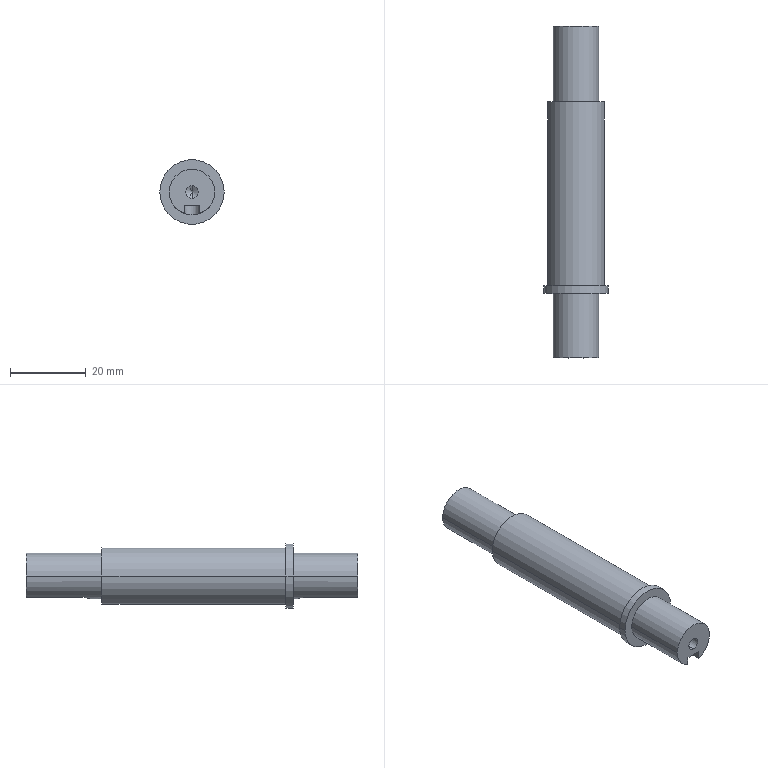Part | SolidWorks | features ICE 3, HoleWzd 2, RefAxis 1, Revolution 1 | 1 solid | 29 faces | box 17 x 87.5 x 17 mm | volume 12724 mm3 | cylinder 14 | plane 11 | cone 4 | commonest cylinder face diameters 3.3 x4 12 x4 4 x2 15 x2 17 x2
STEP:
#1=CARTESIAN_POINT('',(0.,60.4,-1.65));
#2=VERTEX_POINT('',#1);
#3=CARTESIAN_POINT('',(0.,60.4,1.65));
#4=VERTEX_POINT('',#3);
#5=CARTESIAN_POINT('',(0.,60.4,0.));
#6=DIRECTION('',(0.,1.,0.));
#7=DIRECTION('',(0.,0.,1.));
#8=AXIS2_PLACEMENT_3D('',#5,#6,#7);
#9=CIRCLE('',#8,1.65);
#10=EDGE_CURVE('',#2,#4,#9,.T.);
#11=ORIENTED_EDGE('',*,*,#10,.F.);
#12=CARTESIAN_POINT('',(0.,70.5,-1.65));
#13=VERTEX_POINT('',#12);
#14=CARTESIAN_POINT('',(0.,70.5,-1.65));
#15=DIRECTION('',(0.,1.,0.));
#16=VECTOR('',#15,1000.);
#17=LINE('',#14,#16);
#18=EDGE_CURVE('',#2,#13,#17,.T.);
#19=ORIENTED_EDGE('',*,*,#18,.T.);
#20=CARTESIAN_POINT('',(0.,70.5,1.65));
#21=VERTEX_POINT('',#20);
#22=CARTESIAN_POINT('',(0.,70.5,0.));
#23=DIRECTION('',(0.,1.,0.));
#24=DIRECTION('',(0.,0.,1.));
#25=AXIS2_PLACEMENT_3D('',#22,#23,#24);
#26=CIRCLE('',#25,1.65);
#27=EDGE_CURVE('',#13,#21,#26,.T.);
#28=ORIENTED_EDGE('',*,*,#27,.T.);
#29=CARTESIAN_POINT('',(0.,70.5,1.65));
#30=DIRECTION('',(0.,1.,0.));
#31=VECTOR('',#30,1000.);
#32=LINE('',#29,#31);
#33=EDGE_CURVE('',#4,#21,#32,.T.);
#34=ORIENTED_EDGE('',*,*,#33,.F.);
#35=EDGE_LOOP('',(#11,#19,#28,#34));
#36=FACE_OUTER_BOUND('',#35,.T.);
#37=CARTESIAN_POINT('',(0.,70.5,0.));
#38=DIRECTION('',(0.,1.,0.));
#39=DIRECTION('',(0.,0.,1.));
#40=AXIS2_PLACEMENT_3D('',#37,#38,#39);
#41=CYLINDRICAL_SURFACE('',#40,1.65);
#42=ADVANCED_FACE('',(#36),#41,.F.);
#43=CARTESIAN_POINT('',(0.,59.409,0.));
#44=VERTEX_POINT('',#43);
#45=CARTESIAN_POINT('',(0.,60.4,1.65));
#46=DIRECTION('',(0.,0.515,0.8572));
#47=VECTOR('',#46,1000.);
#48=LINE('',#45,#47);
#49=EDGE_CURVE('',#44,#4,#48,.T.);
#50=ORIENTED_EDGE('',*,*,#49,.F.);
#51=CARTESIAN_POINT('',(0.,60.4,-1.65));
#52=DIRECTION('',(0.,0.515,-0.8572));
#53=VECTOR('',#52,1000.);
#54=LINE('',#51,#53);
#55=EDGE_CURVE('',#44,#2,#54,.T.);
#56=ORIENTED_EDGE('',*,*,#55,.T.);
#57=ORIENTED_EDGE('',*,*,#10,.T.);
#58=EDGE_LOOP('',(#50,#56,#57));
#59=FACE_OUTER_BOUND('',#58,.T.);
#60=CARTESIAN_POINT('',(0.,60.4,0.));
#61=DIRECTION('',(0.,1.,0.));
#62=DIRECTION('',(0.,0.,1.));
#63=AXIS2_PLACEMENT_3D('',#60,#61,#62);
#64=CONICAL_SURFACE('',#63,1.65,1.03);
#65=ADVANCED_FACE('',(#59),#64,.F.);
#66=CARTESIAN_POINT('',(0.,-6.9,1.65));
#67=VERTEX_POINT('',#66);
#68=CARTESIAN_POINT('',(0.,-6.9,-1.65));
#69=VERTEX_POINT('',#68);
#70=CARTESIAN_POINT('',(0.,-6.9,0.));
#71=DIRECTION('',(0.,-1.,0.));
#72=DIRECTION('',(0.,0.,-1.));
#73=AXIS2_PLACEMENT_3D('',#70,#71,#72);
#74=CIRCLE('',#73,1.65);
#75=EDGE_CURVE('',#67,#69,#74,.T.);
#76=ORIENTED_EDGE('',*,*,#75,.F.);
#77=CARTESIAN_POINT('',(0.,-17.,1.65));
#78=VERTEX_POINT('',#77);
#79=CARTESIAN_POINT('',(0.,-17.,1.65));
#80=DIRECTION('',(0.,-1.,0.));
#81=VECTOR('',#80,1000.);
#82=LINE('',#79,#81);
#83=EDGE_CURVE('',#67,#78,#82,.T.);
#84=ORIENTED_EDGE('',*,*,#83,.T.);
#85=CARTESIAN_POINT('',(0.,-17.,-1.65));
#86=VERTEX_POINT('',#85);
#87=CARTESIAN_POINT('',(0.,-17.,0.));
#88=DIRECTION('',(0.,-1.,0.));
#89=DIRECTION('',(0.,0.,-1.));
#90=AXIS2_PLACEMENT_3D('',#87,#88,#89);
#91=CIRCLE('',#90,1.65);
#92=EDGE_CURVE('',#78,#86,#91,.T.);
#93=ORIENTED_EDGE('',*,*,#92,.T.);
#94=CARTESIAN_POINT('',(0.,-17.,-1.65));
#95=DIRECTION('',(0.,-1.,0.));
#96=VECTOR('',#95,1000.);
#97=LINE('',#94,#96);
#98=EDGE_CURVE('',#69,#86,#97,.T.);
#99=ORIENTED_EDGE('',*,*,#98,.F.);
#100=EDGE_LOOP('',(#76,#84,#93,#99));
#101=FACE_OUTER_BOUND('',#100,.T.);
#102=CARTESIAN_POINT('',(0.,-17.,0.));
#103=DIRECTION('',(0.,-1.,0.));
#104=DIRECTION('',(0.,0.,-1.));
#105=AXIS2_PLACEMENT_3D('',#102,#103,#104);
#106=CYLINDRICAL_SURFACE('',#105,1.65);
#107=ADVANCED_FACE('',(#101),#106,.F.);
#108=CARTESIAN_POINT('',(0.,-5.909,0.));
#109=VERTEX_POINT('',#108);
#110=CARTESIAN_POINT('',(0.,-6.9,-1.65));
#111=DIRECTION('',(0.,-0.515,-0.8572));
#112=VECTOR('',#111,1000.);
#113=LINE('',#110,#112);
#114=EDGE_CURVE('',#109,#69,#113,.T.);
#115=ORIENTED_EDGE('',*,*,#114,.F.);
#116=CARTESIAN_POINT('',(0.,-6.9,1.65));
#117=DIRECTION('',(0.,-0.515,0.8572));
#118=VECTOR('',#117,1000.);
#119=LINE('',#116,#118);
#120=EDGE_CURVE('',#109,#67,#119,.T.);
#121=ORIENTED_EDGE('',*,*,#120,.T.);
#122=ORIENTED_EDGE('',*,*,#75,.T.);
#123=EDGE_LOOP('',(#115,#121,#122));
#124=FACE_OUTER_BOUND('',#123,.T.);
#125=CARTESIAN_POINT('',(0.,-6.9,0.));
#126=DIRECTION('',(0.,-1.,0.));
#127=DIRECTION('',(0.,0.,-1.));
#128=AXIS2_PLACEMENT_3D('',#125,#126,#127);
#129=CONICAL_SURFACE('',#128,1.65,1.03);
#130=ADVANCED_FACE('',(#124),#129,.F.);
#131=CARTESIAN_POINT('',(6.,-17.,0.));
#132=VERTEX_POINT('',#131);
#133=CARTESIAN_POINT('',(-6.,-17.,0.));
#134=VERTEX_POINT('',#133);
#135=CARTESIAN_POINT('',(0.,-17.,0.));
#136=DIRECTION('',(0.,-1.,0.));
#137=DIRECTION('',(1.,0.,0.));
#138=AXIS2_PLACEMENT_3D('',#135,#136,#137);
#139=CIRCLE('',#138,6.);
#140=EDGE_CURVE('',#132,#134,#139,.T.);
#141=ORIENTED_EDGE('',*,*,#140,.F.);
#142=CARTESIAN_POINT('',(6.,0.,0.));
#143=VERTEX_POINT('',#142);
#144=CARTESIAN_POINT('',(6.,-17.,0.));
#145=DIRECTION('',(0.,1.,0.));
#146=VECTOR('',#145,1000.);
#147=LINE('',#144,#146);
#148=EDGE_CURVE('',#132,#143,#147,.T.);
#149=ORIENTED_EDGE('',*,*,#148,.T.);
#150=CARTESIAN_POINT('',(-6.,0.,0.));
#151=VERTEX_POINT('',#150);
#152=CARTESIAN_POINT('',(0.,0.,0.));
#153=DIRECTION('',(0.,-1.,0.));
#154=DIRECTION('',(1.,0.,0.));
#155=AXIS2_PLACEMENT_3D('',#152,#153,#154);
#156=CIRCLE('',#155,6.);
#157=EDGE_CURVE('',#143,#151,#156,.T.);
#158=ORIENTED_EDGE('',*,*,#157,.T.);
#159=CARTESIAN_POINT('',(-6.,-17.,0.));
#160=DIRECTION('',(0.,1.,0.));
#161=VECTOR('',#160,1000.);
#162=LINE('',#159,#161);
#163=EDGE_CURVE('',#134,#151,#162,.T.);
#164=ORIENTED_EDGE('',*,*,#163,.F.);
#165=EDGE_LOOP('',(#141,#149,#158,#164));
#166=FACE_OUTER_BOUND('',#165,.T.);
#167=CARTESIAN_POINT('',(0.,-17.,0.));
#168=DIRECTION('',(0.,1.,0.));
#169=DIRECTION('',(-1.,0.,0.));
#170=AXIS2_PLACEMENT_3D('',#167,#168,#169);
#171=CYLINDRICAL_SURFACE('',#170,6.);
#172=ADVANCED_FACE('',(#166),#171,.T.);
#173=CARTESIAN_POINT('',(8.5,2.,0.));
#174=VERTEX_POINT('',#173);
#175=CARTESIAN_POINT('',(-8.5,2.,0.));
#176=VERTEX_POINT('',#175);
#177=CARTESIAN_POINT('',(0.,2.,0.));
#178=DIRECTION('',(0.,-1.,0.));
#179=DIRECTION('',(1.,0.,0.));
#180=AXIS2_PLACEMENT_3D('',#177,#178,#179);
#181=CIRCLE('',#180,8.5);
#182=EDGE_CURVE('',#174,#176,#181,.T.);
#183=ORIENTED_EDGE('',*,*,#182,.T.);
#184=CARTESIAN_POINT('',(-8.5,0.,0.));
#185=VERTEX_POINT('',#184);
#186=CARTESIAN_POINT('',(-8.5,0.,0.));
#187=DIRECTION('',(0.,-1.,0.));
#188=VECTOR('',#187,1000.);
#189=LINE('',#186,#188);
#190=EDGE_CURVE('',#176,#185,#189,.T.);
#191=ORIENTED_EDGE('',*,*,#190,.T.);
#192=CARTESIAN_POINT('',(8.5,0.,0.));
#193=VERTEX_POINT('',#192);
#194=CARTESIAN_POINT('',(0.,0.,0.));
#195=DIRECTION('',(0.,-1.,0.));
#196=DIRECTION('',(1.,0.,0.));
#197=AXIS2_PLACEMENT_3D('',#194,#195,#196);
#198=CIRCLE('',#197,8.5);
#199=EDGE_CURVE('',#193,#185,#198,.T.);
#200=ORIENTED_EDGE('',*,*,#199,.F.);
#201=CARTESIAN_POINT('',(8.5,0.,0.));
#202=DIRECTION('',(0.,-1.,0.));
#203=VECTOR('',#202,1000.);
#204=LINE('',#201,#203);
#205=EDGE_CURVE('',#174,#193,#204,.T.);
#206=ORIENTED_EDGE('',*,*,#205,.F.);
#207=EDGE_LOOP('',(#183,#191,#200,#206));
#208=FACE_OUTER_BOUND('',#207,.T.);
#209=CARTESIAN_POINT('',(0.,0.,0.));
#210=DIRECTION('',(0.,-1.,0.));
#211=DIRECTION('',(1.,0.,0.));
#212=AXIS2_PLACEMENT_3D('',#209,#210,#211);
#213=CYLINDRICAL_SURFACE('',#212,8.5);
#214=ADVANCED_FACE('',(#208),#213,.T.);
#215=CARTESIAN_POINT('',(7.5,50.5,0.));
#216=VERTEX_POINT('',#215);
#217=CARTESIAN_POINT('',(-7.5,50.5,0.));
#218=VERTEX_POINT('',#217);
#219=CARTESIAN_POINT('',(0.,50.5,0.));
#220=DIRECTION('',(0.,-1.,0.));
#221=DIRECTION('',(1.,0.,0.));
#222=AXIS2_PLACEMENT_3D('',#219,#220,#221);
#223=CIRCLE('',#222,7.5);
#224=EDGE_CURVE('',#216,#218,#223,.T.);
#225=ORIENTED_EDGE('',*,*,#224,.T.);
#226=CARTESIAN_POINT('',(-7.5,2.,0.));
#227=VERTEX_POINT('',#226);
#228=CARTESIAN_POINT('',(-7.5,0.,0.));
#229=DIRECTION('',(0.,-1.,0.));
#230=VECTOR('',#229,1000.);
#231=LINE('',#228,#230);
#232=EDGE_CURVE('',#218,#227,#231,.T.);
#233=ORIENTED_EDGE('',*,*,#232,.T.);
#234=CARTESIAN_POINT('',(7.5,2.,0.));
#235=VERTEX_POINT('',#234);
#236=CARTESIAN_POINT('',(0.,2.,0.));
#237=DIRECTION('',(0.,-1.,0.));
#238=DIRECTION('',(1.,0.,0.));
#239=AXIS2_PLACEMENT_3D('',#236,#237,#238);
#240=CIRCLE('',#239,7.5);
#241=EDGE_CURVE('',#235,#227,#240,.T.);
#242=ORIENTED_EDGE('',*,*,#241,.F.);
#243=CARTESIAN_POINT('',(7.5,0.,0.));
#244=DIRECTION('',(0.,-1.,0.));
#245=VECTOR('',#244,1000.);
#246=LINE('',#243,#245);
#247=EDGE_CURVE('',#216,#235,#246,.T.);
#248=ORIENTED_EDGE('',*,*,#247,.F.);
#249=EDGE_LOOP('',(#225,#233,#242,#248));
#250=FACE_OUTER_BOUND('',#249,.T.);
#251=CARTESIAN_POINT('',(0.,0.,0.));
#252=DIRECTION('',(0.,-1.,0.));
#253=DIRECTION('',(1.,0.,0.));
#254=AXIS2_PLACEMENT_3D('',#251,#252,#253);
#255=CYLINDRICAL_SURFACE('',#254,7.5);
#256=ADVANCED_FACE('',(#250),#255,.T.);
#257=CARTESIAN_POINT('',(6.,70.5,0.));
#258=VERTEX_POINT('',#257);
#259=CARTESIAN_POINT('',(-6.,70.5,0.));
#260=VERTEX_POINT('',#259);
#261=CARTESIAN_POINT('',(0.,70.5,0.));
#262=DIRECTION('',(0.,-1.,0.));
#263=DIRECTION('',(1.,0.,0.));
#264=AXIS2_PLACEMENT_3D('',#261,#262,#263);
#265=CIRCLE('',#264,6.);
#266=EDGE_CURVE('',#258,#260,#265,.T.);
#267=ORIENTED_EDGE('',*,*,#266,.T.);
#268=CARTESIAN_POINT('',(-6.,50.5,0.));
#269=VERTEX_POINT('',#268);
#270=CARTESIAN_POINT('',(-6.,0.,0.));
#271=DIRECTION('',(0.,-1.,0.));
#272=VECTOR('',#271,1000.);
#273=LINE('',#270,#272);
#274=EDGE_CURVE('',#260,#269,#273,.T.);
#275=ORIENTED_EDGE('',*,*,#274,.T.);
#276=CARTESIAN_POINT('',(6.,50.5,0.));
#277=VERTEX_POINT('',#276);
#278=CARTESIAN_POINT('',(0.,50.5,0.));
#279=DIRECTION('',(0.,-1.,0.));
#280=DIRECTION('',(1.,0.,0.));
#281=AXIS2_PLACEMENT_3D('',#278,#279,#280);
#282=CIRCLE('',#281,6.);
#283=EDGE_CURVE('',#277,#269,#282,.T.);
#284=ORIENTED_EDGE('',*,*,#283,.F.);
#285=CARTESIAN_POINT('',(6.,0.,0.));
#286=DIRECTION('',(0.,-1.,0.));
#287=VECTOR('',#286,1000.);
#288=LINE('',#285,#287);
#289=EDGE_CURVE('',#258,#277,#288,.T.);
#290=ORIENTED_EDGE('',*,*,#289,.F.);
#291=EDGE_LOOP('',(#267,#275,#284,#290));
#292=FACE_OUTER_BOUND('',#291,.T.);
#293=CARTESIAN_POINT('',(0.,0.,0.));
#294=DIRECTION('',(0.,-1.,0.));
#295=DIRECTION('',(1.,0.,0.));
#296=AXIS2_PLACEMENT_3D('',#293,#294,#295);
#297=CYLINDRICAL_SURFACE('',#296,6.);
#298=ADVANCED_FACE('',(#292),#297,.T.);
#299=CARTESIAN_POINT('',(0.,0.,0.));
#300=DIRECTION('',(0.,-1.,0.));
#301=DIRECTION('',(1.,0.,0.));
#302=AXIS2_PLACEMENT_3D('',#299,#300,#301);
#303=CIRCLE('',#302,6.);
#304=EDGE_CURVE('',#151,#143,#303,.T.);
#305=ORIENTED_EDGE('',*,*,#304,.F.);
#306=ORIENTED_EDGE('',*,*,#157,.F.);
#307=EDGE_LOOP('',(#305,#306));
#308=FACE_BOUND('',#307,.T.);
#309=ORIENTED_EDGE('',*,*,#199,.T.);
#310=CARTESIAN_POINT('',(0.,0.,0.));
#311=DIRECTION('',(0.,-1.,0.));
#312=DIRECTION('',(1.,0.,0.));
#313=AXIS2_PLACEMENT_3D('',#310,#311,#312);
#314=CIRCLE('',#313,8.5);
#315=EDGE_CURVE('',#185,#193,#314,.T.);
#316=ORIENTED_EDGE('',*,*,#315,.T.);
#317=EDGE_LOOP('',(#309,#316));
#318=FACE_OUTER_BOUND('',#317,.T.);
#319=CARTESIAN_POINT('',(-8.5,0.,0.));
#320=DIRECTION('',(0.,1.,0.));
#321=DIRECTION('',(-1.,0.,0.));
#322=AXIS2_PLACEMENT_3D('',#319,#320,#321);
#323=PLANE('',#322);
#324=ADVANCED_FACE('',(#308,#318),#323,.F.);
#325=CARTESIAN_POINT('',(0.,70.5,0.));
#326=DIRECTION('',(0.,1.,0.));
#327=DIRECTION('',(0.,0.,1.));
#328=AXIS2_PLACEMENT_3D('',#325,#326,#327);
#329=CIRCLE('',#328,1.65);
#330=EDGE_CURVE('',#21,#13,#329,.T.);
#331=ORIENTED_EDGE('',*,*,#330,.F.);
#332=ORIENTED_EDGE('',*,*,#27,.F.);
#333=EDGE_LOOP('',(#331,#332));
#334=FACE_BOUND('',#333,.T.);
#335=CARTESIAN_POINT('',(-2.,70.5,-3.5));
#336=VERTEX_POINT('',#335);
#337=CARTESIAN_POINT('',(2.,70.5,-3.5));
#338=VERTEX_POINT('',#337);
#339=CARTESIAN_POINT('',(0.,70.5,-3.5));
#340=DIRECTION('',(1.,0.,0.));
#341=VECTOR('',#340,1000.);
#342=LINE('',#339,#341);
#343=EDGE_CURVE('',#336,#338,#342,.T.);
#344=ORIENTED_EDGE('',*,*,#343,.F.);
#345=CARTESIAN_POINT('',(-2.,70.5,-5.657));
#346=VERTEX_POINT('',#345);
#347=CARTESIAN_POINT('',(-2.,70.5,0.));
#348=DIRECTION('',(0.,0.,-1.));
#349=VECTOR('',#348,1000.);
#350=LINE('',#347,#349);
#351=EDGE_CURVE('',#336,#346,#350,.T.);
#352=ORIENTED_EDGE('',*,*,#351,.T.);
#353=CARTESIAN_POINT('',(0.,70.5,0.));
#354=DIRECTION('',(0.,-1.,0.));
#355=DIRECTION('',(1.,0.,0.));
#356=AXIS2_PLACEMENT_3D('',#353,#354,#355);
#357=CIRCLE('',#356,6.);
#358=EDGE_CURVE('',#260,#346,#357,.T.);
#359=ORIENTED_EDGE('',*,*,#358,.F.);
#360=ORIENTED_EDGE('',*,*,#266,.F.);
#361=CARTESIAN_POINT('',(2.,70.5,-5.657));
#362=VERTEX_POINT('',#361);
#363=CARTESIAN_POINT('',(0.,70.5,0.));
#364=DIRECTION('',(0.,-1.,0.));
#365=DIRECTION('',(1.,0.,0.));
#366=AXIS2_PLACEMENT_3D('',#363,#364,#365);
#367=CIRCLE('',#366,6.);
#368=EDGE_CURVE('',#362,#258,#367,.T.);
#369=ORIENTED_EDGE('',*,*,#368,.F.);
#370=CARTESIAN_POINT('',(2.,70.5,0.));
#371=DIRECTION('',(0.,0.,1.));
#372=VECTOR('',#371,1000.);
#373=LINE('',#370,#372);
#374=EDGE_CURVE('',#362,#338,#373,.T.);
#375=ORIENTED_EDGE('',*,*,#374,.T.);
#376=EDGE_LOOP('',(#344,#352,#359,#360,#369,#375));
#377=FACE_OUTER_BOUND('',#376,.T.);
#378=CARTESIAN_POINT('',(0.,70.5,0.));
#379=DIRECTION('',(0.,-1.,0.));
#380=DIRECTION('',(1.,0.,0.));
#381=AXIS2_PLACEMENT_3D('',#378,#379,#380);
#382=PLANE('',#381);
#383=ADVANCED_FACE('',(#334,#377),#382,.F.);
#384=ORIENTED_EDGE('',*,*,#274,.F.);
#385=ORIENTED_EDGE('',*,*,#358,.T.);
#386=CARTESIAN_POINT('',(-2.,55.5,-5.657));
#387=VERTEX_POINT('',#386);
#388=CARTESIAN_POINT('',(-2.,0.,-5.657));
#389=DIRECTION('',(0.,-1.,0.));
#390=VECTOR('',#389,1000.);
#391=LINE('',#388,#390);
#392=EDGE_CURVE('',#346,#387,#391,.T.);
#393=ORIENTED_EDGE('',*,*,#392,.T.);
#394=CARTESIAN_POINT('',(2.,55.5,-5.657));
#395=VERTEX_POINT('',#394);
#396=CARTESIAN_POINT('',(-2.,55.5,-5.657));
#397=CARTESIAN_POINT('',(-2.,55.367,-5.657));
#398=CARTESIAN_POINT('',(-1.987,55.236,-5.662));
#399=CARTESIAN_POINT('',(-1.935,54.979,-5.679));
#400=CARTESIAN_POINT('',(-1.897,54.852,-5.693));
#401=CARTESIAN_POINT('',(-1.796,54.61,-5.725));
#402=CARTESIAN_POINT('',(-1.735,54.496,-5.744));
#403=CARTESIAN_POINT('',(-1.59,54.279,-5.786));
#404=CARTESIAN_POINT('',(-1.506,54.177,-5.809));
#405=CARTESIAN_POINT('',(-1.231,53.903,-5.875));
#406=CARTESIAN_POINT('',(-1.01,53.754,-5.919));
#407=CARTESIAN_POINT('',(-0.6496,53.604,-5.966));
#408=CARTESIAN_POINT('',(-0.5226,53.565,-5.979));
#409=CARTESIAN_POINT('',(-0.264,53.513,-5.996));
#410=CARTESIAN_POINT('',(-0.1336,53.5,-6.));
#411=CARTESIAN_POINT('',(0.1294,53.5,-6.));
#412=CARTESIAN_POINT('',(0.2629,53.513,-5.996));
#413=CARTESIAN_POINT('',(0.5202,53.564,-5.979));
#414=CARTESIAN_POINT('',(0.6454,53.602,-5.966));
#415=CARTESIAN_POINT('',(0.8889,53.704,-5.935));
#416=CARTESIAN_POINT('',(1.004,53.766,-5.916));
#417=CARTESIAN_POINT('',(1.22,53.91,-5.876));
#418=CARTESIAN_POINT('',(1.322,53.993,-5.853));
#419=CARTESIAN_POINT('',(1.506,54.177,-5.809));
#420=CARTESIAN_POINT('',(1.588,54.277,-5.787));
#421=CARTESIAN_POINT('',(1.733,54.493,-5.745));
#422=CARTESIAN_POINT('',(1.796,54.61,-5.725));
#423=CARTESIAN_POINT('',(1.946,54.971,-5.677));
#424=CARTESIAN_POINT('',(2.,55.234,-5.657));
#425=CARTESIAN_POINT('',(2.,55.5,-5.657));
#426=B_SPLINE_CURVE_WITH_KNOTS('',3,(#396,#397,#398,#399,#400,#401,#402,#403,#404,#405,#406,#407,#408,#409,#410,#411,#412,#413,#414,#415,#416,#417,#418,#419,#420,#421,#422,#423,#424,#425),.UNSPECIFIED.,.F.,.F.,(4,2,2,2,2,2,2,2,2,2,2,2,2,2,4),(0.,0.0003935,0.000787,0.00118,0.001574,0.002361,0.002754,0.003148,0.003541,0.003935,0.004328,0.004722,0.005115,0.005509,0.006296),.UNSPECIFIED.);
#427=EDGE_CURVE('',#387,#395,#426,.T.);
#428=ORIENTED_EDGE('',*,*,#427,.T.);
#429=CARTESIAN_POINT('',(2.,0.,-5.657));
#430=DIRECTION('',(0.,1.,0.));
#431=VECTOR('',#430,1000.);
#432=LINE('',#429,#431);
#433=EDGE_CURVE('',#395,#362,#432,.T.);
#434=ORIENTED_EDGE('',*,*,#433,.T.);
#435=ORIENTED_EDGE('',*,*,#368,.T.);
#436=ORIENTED_EDGE('',*,*,#289,.T.);
#437=CARTESIAN_POINT('',(0.,50.5,0.));
#438=DIRECTION('',(0.,-1.,0.));
#439=DIRECTION('',(1.,0.,0.));
#440=AXIS2_PLACEMENT_3D('',#437,#438,#439);
#441=CIRCLE('',#440,6.);
#442=EDGE_CURVE('',#269,#277,#441,.T.);
#443=ORIENTED_EDGE('',*,*,#442,.F.);
#444=EDGE_LOOP('',(#384,#385,#393,#428,#434,#435,#436,#443));
#445=FACE_OUTER_BOUND('',#444,.T.);
#446=CARTESIAN_POINT('',(0.,0.,0.));
#447=DIRECTION('',(0.,-1.,0.));
#448=DIRECTION('',(1.,0.,0.));
#449=AXIS2_PLACEMENT_3D('',#446,#447,#448);
#450=CYLINDRICAL_SURFACE('',#449,6.);
#451=ADVANCED_FACE('',(#445),#450,.T.);
#452=ORIENTED_EDGE('',*,*,#224,.F.);
#453=CARTESIAN_POINT('',(0.,50.5,0.));
#454=DIRECTION('',(0.,-1.,0.));
#455=DIRECTION('',(1.,0.,0.));
#456=AXIS2_PLACEMENT_3D('',#453,#454,#455);
#457=CIRCLE('',#456,7.5);
#458=EDGE_CURVE('',#218,#216,#457,.T.);
#459=ORIENTED_EDGE('',*,*,#458,.F.);
#460=EDGE_LOOP('',(#452,#459));
#461=FACE_OUTER_BOUND('',#460,.T.);
#462=ORIENTED_EDGE('',*,*,#283,.T.);
#463=ORIENTED_EDGE('',*,*,#442,.T.);
#464=EDGE_LOOP('',(#462,#463));
#465=FACE_BOUND('',#464,.T.);
#466=CARTESIAN_POINT('',(-6.,50.5,0.));
#467=DIRECTION('',(0.,-1.,0.));
#468=DIRECTION('',(1.,0.,0.));
#469=AXIS2_PLACEMENT_3D('',#466,#467,#468);
#470=PLANE('',#469);
#471=ADVANCED_FACE('',(#461,#465),#470,.F.);
#472=ORIENTED_EDGE('',*,*,#232,.F.);
#473=ORIENTED_EDGE('',*,*,#458,.T.);
#474=ORIENTED_EDGE('',*,*,#247,.T.);
#475=CARTESIAN_POINT('',(0.,2.,0.));
#476=DIRECTION('',(0.,-1.,0.));
#477=DIRECTION('',(1.,0.,0.));
#478=AXIS2_PLACEMENT_3D('',#475,#476,#477);
#479=CIRCLE('',#478,7.5);
#480=EDGE_CURVE('',#227,#235,#479,.T.);
#481=ORIENTED_EDGE('',*,*,#480,.F.);
#482=EDGE_LOOP('',(#472,#473,#474,#481));
#483=FACE_OUTER_BOUND('',#482,.T.);
#484=CARTESIAN_POINT('',(0.,0.,0.));
#485=DIRECTION('',(0.,-1.,0.));
#486=DIRECTION('',(1.,0.,0.));
#487=AXIS2_PLACEMENT_3D('',#484,#485,#486);
#488=CYLINDRICAL_SURFACE('',#487,7.5);
#489=ADVANCED_FACE('',(#483),#488,.T.);
#490=ORIENTED_EDGE('',*,*,#182,.F.);
#491=CARTESIAN_POINT('',(0.,2.,0.));
#492=DIRECTION('',(0.,-1.,0.));
#493=DIRECTION('',(1.,0.,0.));
#494=AXIS2_PLACEMENT_3D('',#491,#492,#493);
#495=CIRCLE('',#494,8.5);
#496=EDGE_CURVE('',#176,#174,#495,.T.);
#497=ORIENTED_EDGE('',*,*,#496,.F.);
#498=EDGE_LOOP('',(#490,#497));
#499=FACE_OUTER_BOUND('',#498,.T.);
#500=ORIENTED_EDGE('',*,*,#241,.T.);
#501=ORIENTED_EDGE('',*,*,#480,.T.);
#502=EDGE_LOOP('',(#500,#501));
#503=FACE_BOUND('',#502,.T.);
#504=CARTESIAN_POINT('',(-7.5,2.,0.));
#505=DIRECTION('',(0.,-1.,0.));
#506=DIRECTION('',(1.,0.,0.));
#507=AXIS2_PLACEMENT_3D('',#504,#505,#506);
#508=PLANE('',#507);
#509=ADVANCED_FACE('',(#499,#503),#508,.F.);
#510=ORIENTED_EDGE('',*,*,#190,.F.);
#511=ORIENTED_EDGE('',*,*,#496,.T.);
#512=ORIENTED_EDGE('',*,*,#205,.T.);
#513=ORIENTED_EDGE('',*,*,#315,.F.);
#514=EDGE_LOOP('',(#510,#511,#512,#513));
#515=FACE_OUTER_BOUND('',#514,.T.);
#516=CARTESIAN_POINT('',(0.,0.,0.));
#517=DIRECTION('',(0.,-1.,0.));
#518=DIRECTION('',(1.,0.,0.));
#519=AXIS2_PLACEMENT_3D('',#516,#517,#518);
#520=CYLINDRICAL_SURFACE('',#519,8.5);
#521=ADVANCED_FACE('',(#515),#520,.T.);
#522=ORIENTED_EDGE('',*,*,#148,.F.);
#523=CARTESIAN_POINT('',(2.,-17.,-5.657));
#524=VERTEX_POINT('',#523);
#525=CARTESIAN_POINT('',(0.,-17.,0.));
#526=DIRECTION('',(0.,-1.,0.));
#527=DIRECTION('',(1.,0.,0.));
#528=AXIS2_PLACEMENT_3D('',#525,#526,#527);
#529=CIRCLE('',#528,6.);
#530=EDGE_CURVE('',#524,#132,#529,.T.);
#531=ORIENTED_EDGE('',*,*,#530,.F.);
#532=CARTESIAN_POINT('',(2.,-3.,-5.657));
#533=VERTEX_POINT('',#532);
#534=CARTESIAN_POINT('',(2.,-17.,-5.657));
#535=DIRECTION('',(0.,1.,0.));
#536=VECTOR('',#535,1000.);
#537=LINE('',#534,#536);
#538=EDGE_CURVE('',#524,#533,#537,.T.);
#539=ORIENTED_EDGE('',*,*,#538,.T.);
#540=CARTESIAN_POINT('',(-2.,-3.,-5.657));
#541=VERTEX_POINT('',#540);
#542=CARTESIAN_POINT('',(2.,-3.,-5.657));
#543=CARTESIAN_POINT('',(2.,-2.867,-5.657));
#544=CARTESIAN_POINT('',(1.987,-2.736,-5.662));
#545=CARTESIAN_POINT('',(1.935,-2.479,-5.679));
#546=CARTESIAN_POINT('',(1.897,-2.352,-5.693));
#547=CARTESIAN_POINT('',(1.796,-2.11,-5.725));
#548=CARTESIAN_POINT('',(1.735,-1.996,-5.744));
#549=CARTESIAN_POINT('',(1.59,-1.779,-5.786));
#550=CARTESIAN_POINT('',(1.506,-1.677,-5.809));
#551=CARTESIAN_POINT('',(1.231,-1.403,-5.875));
#552=CARTESIAN_POINT('',(1.01,-1.254,-5.919));
#553=CARTESIAN_POINT('',(0.6496,-1.104,-5.966));
#554=CARTESIAN_POINT('',(0.5226,-1.065,-5.979));
#555=CARTESIAN_POINT('',(0.264,-1.013,-5.996));
#556=CARTESIAN_POINT('',(0.1336,-1.,-6.));
#557=CARTESIAN_POINT('',(-0.1294,-0.9999,-6.));
#558=CARTESIAN_POINT('',(-0.2629,-1.013,-5.996));
#559=CARTESIAN_POINT('',(-0.5202,-1.064,-5.979));
#560=CARTESIAN_POINT('',(-0.6454,-1.102,-5.966));
#561=CARTESIAN_POINT('',(-0.8889,-1.204,-5.935));
#562=CARTESIAN_POINT('',(-1.004,-1.266,-5.916));
#563=CARTESIAN_POINT('',(-1.22,-1.41,-5.876));
#564=CARTESIAN_POINT('',(-1.322,-1.493,-5.853));
#565=CARTESIAN_POINT('',(-1.506,-1.677,-5.809));
#566=CARTESIAN_POINT('',(-1.588,-1.777,-5.787));
#567=CARTESIAN_POINT('',(-1.733,-1.993,-5.745));
#568=CARTESIAN_POINT('',(-1.796,-2.11,-5.725));
#569=CARTESIAN_POINT('',(-1.946,-2.471,-5.677));
#570=CARTESIAN_POINT('',(-2.,-2.734,-5.657));
#571=CARTESIAN_POINT('',(-2.,-3.,-5.657));
#572=B_SPLINE_CURVE_WITH_KNOTS('',3,(#542,#543,#544,#545,#546,#547,#548,#549,#550,#551,#552,#553,#554,#555,#556,#557,#558,#559,#560,#561,#562,#563,#564,#565,#566,#567,#568,#569,#570,#571),.UNSPECIFIED.,.F.,.F.,(4,2,2,2,2,2,2,2,2,2,2,2,2,2,4),(0.,0.0003935,0.000787,0.00118,0.001574,0.002361,0.002754,0.003148,0.003541,0.003935,0.004328,0.004722,0.005115,0.005509,0.006296),.UNSPECIFIED.);
#573=EDGE_CURVE('',#533,#541,#572,.T.);
#574=ORIENTED_EDGE('',*,*,#573,.T.);
#575=CARTESIAN_POINT('',(-2.,-17.,-5.657));
#576=VERTEX_POINT('',#575);
#577=CARTESIAN_POINT('',(-2.,-17.,-5.657));
#578=DIRECTION('',(0.,-1.,0.));
#579=VECTOR('',#578,1000.);
#580=LINE('',#577,#579);
#581=EDGE_CURVE('',#541,#576,#580,.T.);
#582=ORIENTED_EDGE('',*,*,#581,.T.);
#583=CARTESIAN_POINT('',(0.,-17.,0.));
#584=DIRECTION('',(0.,-1.,0.));
#585=DIRECTION('',(1.,0.,0.));
#586=AXIS2_PLACEMENT_3D('',#583,#584,#585);
#587=CIRCLE('',#586,6.);
#588=EDGE_CURVE('',#134,#576,#587,.T.);
#589=ORIENTED_EDGE('',*,*,#588,.F.);
#590=ORIENTED_EDGE('',*,*,#163,.T.);
#591=ORIENTED_EDGE('',*,*,#304,.T.);
#592=EDGE_LOOP('',(#522,#531,#539,#574,#582,#589,#590,#591));
#593=FACE_OUTER_BOUND('',#592,.T.);
#594=CARTESIAN_POINT('',(0.,-17.,0.));
#595=DIRECTION('',(0.,1.,0.));
#596=DIRECTION('',(-1.,0.,0.));
#597=AXIS2_PLACEMENT_3D('',#594,#595,#596);
#598=CYLINDRICAL_SURFACE('',#597,6.);
#599=ADVANCED_FACE('',(#593),#598,.T.);
#600=CARTESIAN_POINT('',(0.,-17.,0.));
#601=DIRECTION('',(0.,-1.,0.));
#602=DIRECTION('',(0.,0.,-1.));
#603=AXIS2_PLACEMENT_3D('',#600,#601,#602);
#604=CIRCLE('',#603,1.65);
#605=EDGE_CURVE('',#86,#78,#604,.T.);
#606=ORIENTED_EDGE('',*,*,#605,.F.);
#607=ORIENTED_EDGE('',*,*,#92,.F.);
#608=EDGE_LOOP('',(#606,#607));
#609=FACE_BOUND('',#608,.T.);
#610=CARTESIAN_POINT('',(2.,-17.,-3.5));
#611=VERTEX_POINT('',#610);
#612=CARTESIAN_POINT('',(2.,-17.,0.));
#613=DIRECTION('',(0.,0.,1.));
#614=VECTOR('',#613,1000.);
#615=LINE('',#612,#614);
#616=EDGE_CURVE('',#524,#611,#615,.T.);
#617=ORIENTED_EDGE('',*,*,#616,.F.);
#618=ORIENTED_EDGE('',*,*,#530,.T.);
#619=ORIENTED_EDGE('',*,*,#140,.T.);
#620=ORIENTED_EDGE('',*,*,#588,.T.);
#621=CARTESIAN_POINT('',(-2.,-17.,-3.5));
#622=VERTEX_POINT('',#621);
#623=CARTESIAN_POINT('',(-2.,-17.,0.));
#624=DIRECTION('',(0.,0.,-1.));
#625=VECTOR('',#624,1000.);
#626=LINE('',#623,#625);
#627=EDGE_CURVE('',#622,#576,#626,.T.);
#628=ORIENTED_EDGE('',*,*,#627,.F.);
#629=CARTESIAN_POINT('',(0.,-17.,-3.5));
#630=DIRECTION('',(1.,0.,0.));
#631=VECTOR('',#630,1000.);
#632=LINE('',#629,#631);
#633=EDGE_CURVE('',#622,#611,#632,.T.);
#634=ORIENTED_EDGE('',*,*,#633,.T.);
#635=EDGE_LOOP('',(#617,#618,#619,#620,#628,#634));
#636=FACE_OUTER_BOUND('',#635,.T.);
#637=CARTESIAN_POINT('',(0.,-17.,0.));
#638=DIRECTION('',(0.,-1.,0.));
#639=DIRECTION('',(1.,0.,0.));
#640=AXIS2_PLACEMENT_3D('',#637,#638,#639);
#641=PLANE('',#640);
#642=ADVANCED_FACE('',(#609,#636),#641,.T.);
#643=ORIENTED_EDGE('',*,*,#343,.T.);
#644=CARTESIAN_POINT('',(2.,55.5,-3.5));
#645=VERTEX_POINT('',#644);
#646=CARTESIAN_POINT('',(2.,71.5,-3.5));
#647=DIRECTION('',(0.,-1.,0.));
#648=VECTOR('',#647,1000.);
#649=LINE('',#646,#648);
#650=EDGE_CURVE('',#338,#645,#649,.T.);
#651=ORIENTED_EDGE('',*,*,#650,.T.);
#652=CARTESIAN_POINT('',(-2.,55.5,-3.5));
#653=VERTEX_POINT('',#652);
#654=CARTESIAN_POINT('',(0.,55.5,-3.5));
#655=DIRECTION('',(0.,0.,-1.));
#656=DIRECTION('',(-1.,0.,0.));
#657=AXIS2_PLACEMENT_3D('',#654,#655,#656);
#658=CIRCLE('',#657,2.);
#659=EDGE_CURVE('',#645,#653,#658,.T.);
#660=ORIENTED_EDGE('',*,*,#659,.T.);
#661=CARTESIAN_POINT('',(-2.,71.5,-3.5));
#662=DIRECTION('',(0.,1.,0.));
#663=VECTOR('',#662,1000.);
#664=LINE('',#661,#663);
#665=EDGE_CURVE('',#653,#336,#664,.T.);
#666=ORIENTED_EDGE('',*,*,#665,.T.);
#667=EDGE_LOOP('',(#643,#651,#660,#666));
#668=FACE_OUTER_BOUND('',#667,.T.);
#669=CARTESIAN_POINT('',(0.,71.5,-3.5));
#670=DIRECTION('',(0.,0.,-1.));
#671=DIRECTION('',(-1.,0.,0.));
#672=AXIS2_PLACEMENT_3D('',#669,#670,#671);
#673=PLANE('',#672);
#674=ADVANCED_FACE('',(#668),#673,.T.);
#675=ORIENTED_EDGE('',*,*,#665,.F.);
#676=CARTESIAN_POINT('',(-2.,55.5,-3.5));
#677=DIRECTION('',(0.,0.,-1.));
#678=VECTOR('',#677,1000.);
#679=LINE('',#676,#678);
#680=EDGE_CURVE('',#653,#387,#679,.T.);
#681=ORIENTED_EDGE('',*,*,#680,.T.);
#682=ORIENTED_EDGE('',*,*,#392,.F.);
#683=ORIENTED_EDGE('',*,*,#351,.F.);
#684=EDGE_LOOP('',(#675,#681,#682,#683));
#685=FACE_OUTER_BOUND('',#684,.T.);
#686=CARTESIAN_POINT('',(-2.,71.5,-3.5));
#687=DIRECTION('',(-1.,0.,0.));
#688=DIRECTION('',(0.,0.,1.));
#689=AXIS2_PLACEMENT_3D('',#686,#687,#688);
#690=PLANE('',#689);
#691=ADVANCED_FACE('',(#685),#690,.F.);
#692=ORIENTED_EDGE('',*,*,#680,.F.);
#693=ORIENTED_EDGE('',*,*,#659,.F.);
#694=CARTESIAN_POINT('',(2.,55.5,-3.5));
#695=DIRECTION('',(0.,0.,-1.));
#696=VECTOR('',#695,1000.);
#697=LINE('',#694,#696);
#698=EDGE_CURVE('',#645,#395,#697,.T.);
#699=ORIENTED_EDGE('',*,*,#698,.T.);
#700=ORIENTED_EDGE('',*,*,#427,.F.);
#701=EDGE_LOOP('',(#692,#693,#699,#700));
#702=FACE_OUTER_BOUND('',#701,.T.);
#703=CARTESIAN_POINT('',(0.,55.5,-3.5));
#704=DIRECTION('',(0.,0.,-1.));
#705=DIRECTION('',(-1.,0.,0.));
#706=AXIS2_PLACEMENT_3D('',#703,#704,#705);
#707=CYLINDRICAL_SURFACE('',#706,2.);
#708=ADVANCED_FACE('',(#702),#707,.F.);
#709=ORIENTED_EDGE('',*,*,#433,.F.);
#710=ORIENTED_EDGE('',*,*,#698,.F.);
#711=ORIENTED_EDGE('',*,*,#650,.F.);
#712=ORIENTED_EDGE('',*,*,#374,.F.);
#713=EDGE_LOOP('',(#709,#710,#711,#712));
#714=FACE_OUTER_BOUND('',#713,.T.);
#715=CARTESIAN_POINT('',(2.,71.5,-3.5));
#716=DIRECTION('',(1.,0.,0.));
#717=DIRECTION('',(0.,0.,-1.));
#718=AXIS2_PLACEMENT_3D('',#715,#716,#717);
#719=PLANE('',#718);
#720=ADVANCED_FACE('',(#714),#719,.F.);
#721=CARTESIAN_POINT('',(2.,-3.,-3.5));
#722=VERTEX_POINT('',#721);
#723=CARTESIAN_POINT('',(2.,-3.,-3.5));
#724=DIRECTION('',(0.,0.,-1.));
#725=VECTOR('',#724,1000.);
#726=LINE('',#723,#725);
#727=EDGE_CURVE('',#722,#533,#726,.T.);
#728=ORIENTED_EDGE('',*,*,#727,.F.);
#729=CARTESIAN_POINT('',(-2.,-3.,-3.5));
#730=VERTEX_POINT('',#729);
#731=CARTESIAN_POINT('',(0.,-3.,-3.5));
#732=DIRECTION('',(0.,0.,-1.));
#733=DIRECTION('',(-1.,0.,0.));
#734=AXIS2_PLACEMENT_3D('',#731,#732,#733);
#735=CIRCLE('',#734,2.);
#736=EDGE_CURVE('',#730,#722,#735,.T.);
#737=ORIENTED_EDGE('',*,*,#736,.F.);
#738=CARTESIAN_POINT('',(-2.,-3.,-3.5));
#739=DIRECTION('',(0.,0.,-1.));
#740=VECTOR('',#739,1000.);
#741=LINE('',#738,#740);
#742=EDGE_CURVE('',#730,#541,#741,.T.);
#743=ORIENTED_EDGE('',*,*,#742,.T.);
#744=ORIENTED_EDGE('',*,*,#573,.F.);
#745=EDGE_LOOP('',(#728,#737,#743,#744));
#746=FACE_OUTER_BOUND('',#745,.T.);
#747=CARTESIAN_POINT('',(0.,-3.,-3.5));
#748=DIRECTION('',(0.,0.,-1.));
#749=DIRECTION('',(-1.,0.,0.));
#750=AXIS2_PLACEMENT_3D('',#747,#748,#749);
#751=CYLINDRICAL_SURFACE('',#750,2.);
#752=ADVANCED_FACE('',(#746),#751,.F.);
#753=ORIENTED_EDGE('',*,*,#616,.T.);
#754=CARTESIAN_POINT('',(2.,-18.,-3.5));
#755=DIRECTION('',(0.,-1.,0.));
#756=VECTOR('',#755,1000.);
#757=LINE('',#754,#756);
#758=EDGE_CURVE('',#722,#611,#757,.T.);
#759=ORIENTED_EDGE('',*,*,#758,.F.);
#760=ORIENTED_EDGE('',*,*,#727,.T.);
#761=ORIENTED_EDGE('',*,*,#538,.F.);
#762=EDGE_LOOP('',(#753,#759,#760,#761));
#763=FACE_OUTER_BOUND('',#762,.T.);
#764=CARTESIAN_POINT('',(2.,-18.,-3.5));
#765=DIRECTION('',(1.,0.,0.));
#766=DIRECTION('',(0.,0.,-1.));
#767=AXIS2_PLACEMENT_3D('',#764,#765,#766);
#768=PLANE('',#767);
#769=ADVANCED_FACE('',(#763),#768,.F.);
#770=ORIENTED_EDGE('',*,*,#742,.F.);
#771=CARTESIAN_POINT('',(-2.,-18.,-3.5));
#772=DIRECTION('',(0.,1.,0.));
#773=VECTOR('',#772,1000.);
#774=LINE('',#771,#773);
#775=EDGE_CURVE('',#622,#730,#774,.T.);
#776=ORIENTED_EDGE('',*,*,#775,.F.);
#777=ORIENTED_EDGE('',*,*,#627,.T.);
#778=ORIENTED_EDGE('',*,*,#581,.F.);
#779=EDGE_LOOP('',(#770,#776,#777,#778));
#780=FACE_OUTER_BOUND('',#779,.T.);
#781=CARTESIAN_POINT('',(-2.,-18.,-3.5));
#782=DIRECTION('',(-1.,0.,0.));
#783=DIRECTION('',(0.,0.,1.));
#784=AXIS2_PLACEMENT_3D('',#781,#782,#783);
#785=PLANE('',#784);
#786=ADVANCED_FACE('',(#780),#785,.F.);
#787=ORIENTED_EDGE('',*,*,#775,.T.);
#788=ORIENTED_EDGE('',*,*,#736,.T.);
#789=ORIENTED_EDGE('',*,*,#758,.T.);
#790=ORIENTED_EDGE('',*,*,#633,.F.);
#791=EDGE_LOOP('',(#787,#788,#789,#790));
#792=FACE_OUTER_BOUND('',#791,.T.);
#793=CARTESIAN_POINT('',(0.,-18.,-3.5));
#794=DIRECTION('',(0.,0.,-1.));
#795=DIRECTION('',(-1.,0.,0.));
#796=AXIS2_PLACEMENT_3D('',#793,#794,#795);
#797=PLANE('',#796);
#798=ADVANCED_FACE('',(#792),#797,.T.);
#799=ORIENTED_EDGE('',*,*,#120,.F.);
#800=ORIENTED_EDGE('',*,*,#114,.T.);
#801=CARTESIAN_POINT('',(0.,-6.9,0.));
#802=DIRECTION('',(0.,-1.,0.));
#803=DIRECTION('',(0.,0.,-1.));
#804=AXIS2_PLACEMENT_3D('',#801,#802,#803);
#805=CIRCLE('',#804,1.65);
#806=EDGE_CURVE('',#69,#67,#805,.T.);
#807=ORIENTED_EDGE('',*,*,#806,.T.);
#808=EDGE_LOOP('',(#799,#800,#807));
#809=FACE_OUTER_BOUND('',#808,.T.);
#810=CARTESIAN_POINT('',(0.,-6.9,0.));
#811=DIRECTION('',(0.,-1.,0.));
#812=DIRECTION('',(0.,0.,-1.));
#813=AXIS2_PLACEMENT_3D('',#810,#811,#812);
#814=CONICAL_SURFACE('',#813,1.65,1.03);
#815=ADVANCED_FACE('',(#809),#814,.F.);
#816=ORIENTED_EDGE('',*,*,#83,.F.);
#817=ORIENTED_EDGE('',*,*,#806,.F.);
#818=ORIENTED_EDGE('',*,*,#98,.T.);
#819=ORIENTED_EDGE('',*,*,#605,.T.);
#820=EDGE_LOOP('',(#816,#817,#818,#819));
#821=FACE_OUTER_BOUND('',#820,.T.);
#822=CARTESIAN_POINT('',(0.,-17.,0.));
#823=DIRECTION('',(0.,-1.,0.));
#824=DIRECTION('',(0.,0.,-1.));
#825=AXIS2_PLACEMENT_3D('',#822,#823,#824);
#826=CYLINDRICAL_SURFACE('',#825,1.65);
#827=ADVANCED_FACE('',(#821),#826,.F.);
#828=ORIENTED_EDGE('',*,*,#55,.F.);
#829=ORIENTED_EDGE('',*,*,#49,.T.);
#830=CARTESIAN_POINT('',(0.,60.4,0.));
#831=DIRECTION('',(0.,1.,0.));
#832=DIRECTION('',(0.,0.,1.));
#833=AXIS2_PLACEMENT_3D('',#830,#831,#832);
#834=CIRCLE('',#833,1.65);
#835=EDGE_CURVE('',#4,#2,#834,.T.);
#836=ORIENTED_EDGE('',*,*,#835,.T.);
#837=EDGE_LOOP('',(#828,#829,#836));
#838=FACE_OUTER_BOUND('',#837,.T.);
#839=CARTESIAN_POINT('',(0.,60.4,0.));
#840=DIRECTION('',(0.,1.,0.));
#841=DIRECTION('',(0.,0.,1.));
#842=AXIS2_PLACEMENT_3D('',#839,#840,#841);
#843=CONICAL_SURFACE('',#842,1.65,1.03);
#844=ADVANCED_FACE('',(#838),#843,.F.);
#845=ORIENTED_EDGE('',*,*,#18,.F.);
#846=ORIENTED_EDGE('',*,*,#835,.F.);
#847=ORIENTED_EDGE('',*,*,#33,.T.);
#848=ORIENTED_EDGE('',*,*,#330,.T.);
#849=EDGE_LOOP('',(#845,#846,#847,#848));
#850=FACE_OUTER_BOUND('',#849,.T.);
#851=CARTESIAN_POINT('',(0.,70.5,0.));
#852=DIRECTION('',(0.,1.,0.));
#853=DIRECTION('',(0.,0.,1.));
#854=AXIS2_PLACEMENT_3D('',#851,#852,#853);
#855=CYLINDRICAL_SURFACE('',#854,1.65);
#856=ADVANCED_FACE('',(#850),#855,.F.);
#857=CLOSED_SHELL('',(#42,#65,#107,#130,#172,#214,#256,#298,#324,#383,#451,#471,#489,#509,#521,#599,#642,#674,#691,#708,#720,#752,#769,#786,#798,#815,#827,#844,#856));
#858=MANIFOLD_SOLID_BREP('',#857);
#859=CARTESIAN_POINT('',(0.,0.,0.));
#860=DIRECTION('',(0.,0.,1.));
#861=DIRECTION('',(1.,0.,0.));
#862=AXIS2_PLACEMENT_3D('',#859,#860,#861);
#863=(LENGTH_UNIT()NAMED_UNIT(*)SI_UNIT(.MILLI.,.METRE.));
#864=UNCERTAINTY_MEASURE_WITH_UNIT(LENGTH_MEASURE(0.00001),#863,'','');
#865=(NAMED_UNIT(*)PLANE_ANGLE_UNIT()SI_UNIT($,.RADIAN.));
#866=(NAMED_UNIT(*)SI_UNIT($,.STERADIAN.)SOLID_ANGLE_UNIT());
#867=(GEOMETRIC_REPRESENTATION_CONTEXT(3)GLOBAL_UNCERTAINTY_ASSIGNED_CONTEXT((#864))GLOBAL_UNIT_ASSIGNED_CONTEXT((#863,#865,#866))REPRESENTATION_CONTEXT('',''));
#868=ADVANCED_BREP_SHAPE_REPRESENTATION('',(#858,#862),#867);